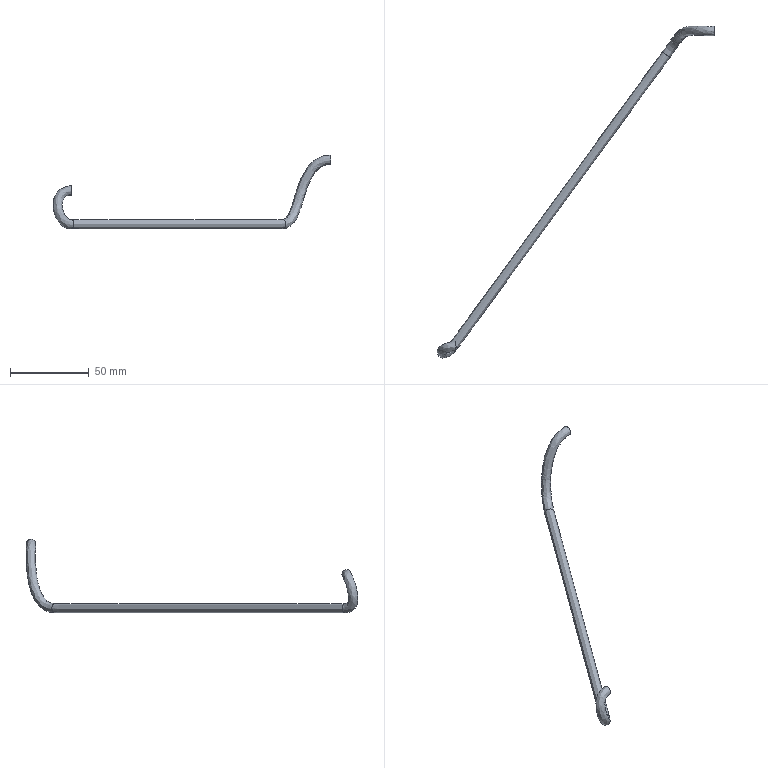Part | NX | features solid 2 | 1 solid | 8 faces | box 176.978 x 211.426 x 47.002 mm | volume 5079 mm3 | spline 6 | plane 2